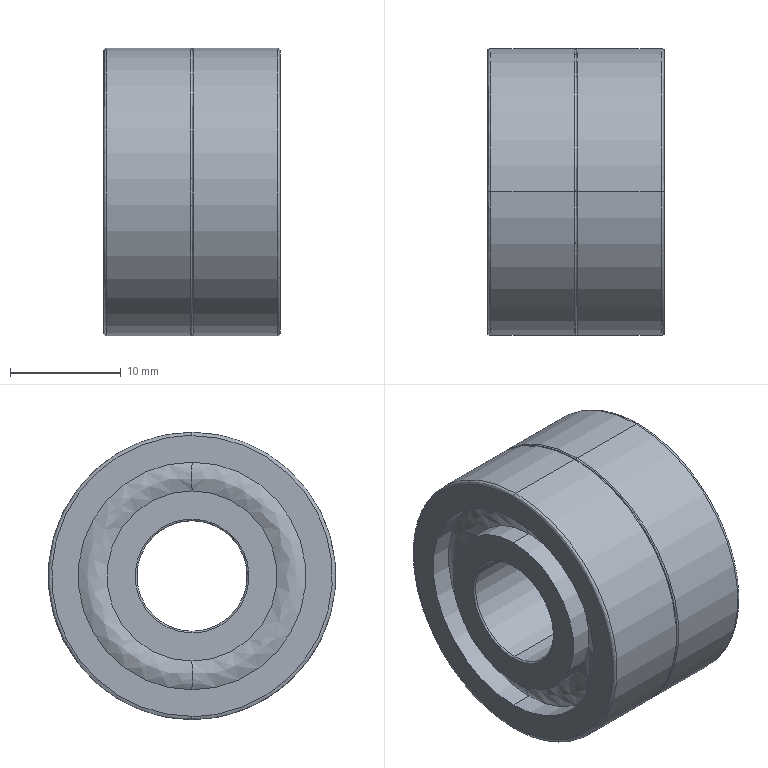Part | SolidWorks | features BaseBody 1 | 1 solid | 40 faces | box 16 x 26 x 26 mm | volume 6727 mm3 | spline 20 | cylinder 16 | plane 4 | commonest cylinder face diameters 10 x4 15.4 x4 20.6 x4 26 x4